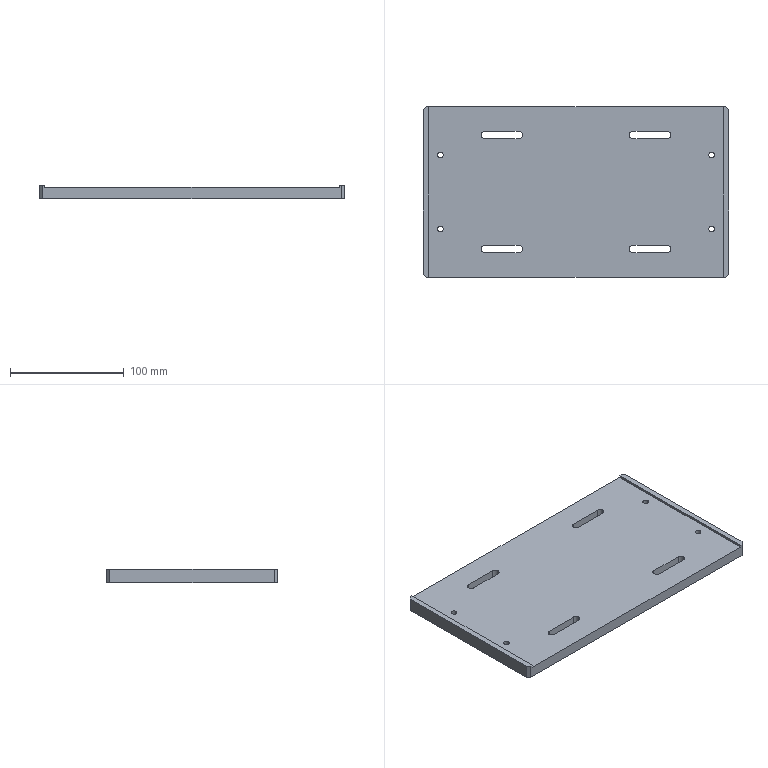Part | SolidWorks | features ICE 2, Chamfer 1, Extrusion 1, HoleWzd 1 | 1 solid | 42 faces | box 268 x 150 x 12 mm | volume 394710 mm3 | plane 22 | cylinder 20 | commonest cylinder face diameters 6.6 x12 5 x8
STEP:
#1=CARTESIAN_POINT('',(-121.5,32.5,0.));
#2=VERTEX_POINT('',#1);
#3=CARTESIAN_POINT('',(-116.5,32.5,0.));
#4=VERTEX_POINT('',#3);
#5=CARTESIAN_POINT('',(-119.,32.5,0.));
#6=DIRECTION('',(0.,0.,1.));
#7=DIRECTION('',(1.,0.,0.));
#8=AXIS2_PLACEMENT_3D('',#5,#6,#7);
#9=CIRCLE('',#8,2.5);
#10=EDGE_CURVE('',#2,#4,#9,.T.);
#11=ORIENTED_EDGE('',*,*,#10,.F.);
#12=CARTESIAN_POINT('',(-121.5,32.5,10.));
#13=VERTEX_POINT('',#12);
#14=CARTESIAN_POINT('',(-121.5,32.5,10.));
#15=DIRECTION('',(0.,0.,1.));
#16=VECTOR('',#15,1000.);
#17=LINE('',#14,#16);
#18=EDGE_CURVE('',#2,#13,#17,.T.);
#19=ORIENTED_EDGE('',*,*,#18,.T.);
#20=CARTESIAN_POINT('',(-116.5,32.5,10.));
#21=VERTEX_POINT('',#20);
#22=CARTESIAN_POINT('',(-119.,32.5,10.));
#23=DIRECTION('',(0.,0.,1.));
#24=DIRECTION('',(1.,0.,0.));
#25=AXIS2_PLACEMENT_3D('',#22,#23,#24);
#26=CIRCLE('',#25,2.5);
#27=EDGE_CURVE('',#13,#21,#26,.T.);
#28=ORIENTED_EDGE('',*,*,#27,.T.);
#29=CARTESIAN_POINT('',(-116.5,32.5,10.));
#30=DIRECTION('',(0.,0.,1.));
#31=VECTOR('',#30,1000.);
#32=LINE('',#29,#31);
#33=EDGE_CURVE('',#4,#21,#32,.T.);
#34=ORIENTED_EDGE('',*,*,#33,.F.);
#35=EDGE_LOOP('',(#11,#19,#28,#34));
#36=FACE_OUTER_BOUND('',#35,.T.);
#37=CARTESIAN_POINT('',(-119.,32.5,10.));
#38=DIRECTION('',(0.,0.,1.));
#39=DIRECTION('',(1.,0.,0.));
#40=AXIS2_PLACEMENT_3D('',#37,#38,#39);
#41=CYLINDRICAL_SURFACE('',#40,2.5);
#42=ADVANCED_FACE('',(#36),#41,.F.);
#43=CARTESIAN_POINT('',(-121.5,-32.5,0.));
#44=VERTEX_POINT('',#43);
#45=CARTESIAN_POINT('',(-116.5,-32.5,0.));
#46=VERTEX_POINT('',#45);
#47=CARTESIAN_POINT('',(-119.,-32.5,0.));
#48=DIRECTION('',(0.,0.,1.));
#49=DIRECTION('',(1.,0.,0.));
#50=AXIS2_PLACEMENT_3D('',#47,#48,#49);
#51=CIRCLE('',#50,2.5);
#52=EDGE_CURVE('',#44,#46,#51,.T.);
#53=ORIENTED_EDGE('',*,*,#52,.F.);
#54=CARTESIAN_POINT('',(-121.5,-32.5,10.));
#55=VERTEX_POINT('',#54);
#56=CARTESIAN_POINT('',(-121.5,-32.5,10.));
#57=DIRECTION('',(0.,0.,1.));
#58=VECTOR('',#57,1000.);
#59=LINE('',#56,#58);
#60=EDGE_CURVE('',#44,#55,#59,.T.);
#61=ORIENTED_EDGE('',*,*,#60,.T.);
#62=CARTESIAN_POINT('',(-116.5,-32.5,10.));
#63=VERTEX_POINT('',#62);
#64=CARTESIAN_POINT('',(-119.,-32.5,10.));
#65=DIRECTION('',(0.,0.,1.));
#66=DIRECTION('',(1.,0.,0.));
#67=AXIS2_PLACEMENT_3D('',#64,#65,#66);
#68=CIRCLE('',#67,2.5);
#69=EDGE_CURVE('',#55,#63,#68,.T.);
#70=ORIENTED_EDGE('',*,*,#69,.T.);
#71=CARTESIAN_POINT('',(-116.5,-32.5,10.));
#72=DIRECTION('',(0.,0.,1.));
#73=VECTOR('',#72,1000.);
#74=LINE('',#71,#73);
#75=EDGE_CURVE('',#46,#63,#74,.T.);
#76=ORIENTED_EDGE('',*,*,#75,.F.);
#77=EDGE_LOOP('',(#53,#61,#70,#76));
#78=FACE_OUTER_BOUND('',#77,.T.);
#79=CARTESIAN_POINT('',(-119.,-32.5,10.));
#80=DIRECTION('',(0.,0.,1.));
#81=DIRECTION('',(1.,0.,0.));
#82=AXIS2_PLACEMENT_3D('',#79,#80,#81);
#83=CYLINDRICAL_SURFACE('',#82,2.5);
#84=ADVANCED_FACE('',(#78),#83,.F.);
#85=CARTESIAN_POINT('',(116.5,32.5,0.));
#86=VERTEX_POINT('',#85);
#87=CARTESIAN_POINT('',(121.5,32.5,0.));
#88=VERTEX_POINT('',#87);
#89=CARTESIAN_POINT('',(119.,32.5,0.));
#90=DIRECTION('',(0.,0.,1.));
#91=DIRECTION('',(1.,0.,0.));
#92=AXIS2_PLACEMENT_3D('',#89,#90,#91);
#93=CIRCLE('',#92,2.5);
#94=EDGE_CURVE('',#86,#88,#93,.T.);
#95=ORIENTED_EDGE('',*,*,#94,.F.);
#96=CARTESIAN_POINT('',(116.5,32.5,10.));
#97=VERTEX_POINT('',#96);
#98=CARTESIAN_POINT('',(116.5,32.5,10.));
#99=DIRECTION('',(0.,0.,1.));
#100=VECTOR('',#99,1000.);
#101=LINE('',#98,#100);
#102=EDGE_CURVE('',#86,#97,#101,.T.);
#103=ORIENTED_EDGE('',*,*,#102,.T.);
#104=CARTESIAN_POINT('',(121.5,32.5,10.));
#105=VERTEX_POINT('',#104);
#106=CARTESIAN_POINT('',(119.,32.5,10.));
#107=DIRECTION('',(0.,0.,1.));
#108=DIRECTION('',(1.,0.,0.));
#109=AXIS2_PLACEMENT_3D('',#106,#107,#108);
#110=CIRCLE('',#109,2.5);
#111=EDGE_CURVE('',#97,#105,#110,.T.);
#112=ORIENTED_EDGE('',*,*,#111,.T.);
#113=CARTESIAN_POINT('',(121.5,32.5,10.));
#114=DIRECTION('',(0.,0.,1.));
#115=VECTOR('',#114,1000.);
#116=LINE('',#113,#115);
#117=EDGE_CURVE('',#88,#105,#116,.T.);
#118=ORIENTED_EDGE('',*,*,#117,.F.);
#119=EDGE_LOOP('',(#95,#103,#112,#118));
#120=FACE_OUTER_BOUND('',#119,.T.);
#121=CARTESIAN_POINT('',(119.,32.5,10.));
#122=DIRECTION('',(0.,0.,1.));
#123=DIRECTION('',(1.,0.,0.));
#124=AXIS2_PLACEMENT_3D('',#121,#122,#123);
#125=CYLINDRICAL_SURFACE('',#124,2.5);
#126=ADVANCED_FACE('',(#120),#125,.F.);
#127=CARTESIAN_POINT('',(116.5,-32.5,0.));
#128=VERTEX_POINT('',#127);
#129=CARTESIAN_POINT('',(121.5,-32.5,0.));
#130=VERTEX_POINT('',#129);
#131=CARTESIAN_POINT('',(119.,-32.5,0.));
#132=DIRECTION('',(0.,0.,1.));
#133=DIRECTION('',(1.,0.,0.));
#134=AXIS2_PLACEMENT_3D('',#131,#132,#133);
#135=CIRCLE('',#134,2.5);
#136=EDGE_CURVE('',#128,#130,#135,.T.);
#137=ORIENTED_EDGE('',*,*,#136,.F.);
#138=CARTESIAN_POINT('',(116.5,-32.5,10.));
#139=VERTEX_POINT('',#138);
#140=CARTESIAN_POINT('',(116.5,-32.5,10.));
#141=DIRECTION('',(0.,0.,1.));
#142=VECTOR('',#141,1000.);
#143=LINE('',#140,#142);
#144=EDGE_CURVE('',#128,#139,#143,.T.);
#145=ORIENTED_EDGE('',*,*,#144,.T.);
#146=CARTESIAN_POINT('',(121.5,-32.5,10.));
#147=VERTEX_POINT('',#146);
#148=CARTESIAN_POINT('',(119.,-32.5,10.));
#149=DIRECTION('',(0.,0.,1.));
#150=DIRECTION('',(1.,0.,0.));
#151=AXIS2_PLACEMENT_3D('',#148,#149,#150);
#152=CIRCLE('',#151,2.5);
#153=EDGE_CURVE('',#139,#147,#152,.T.);
#154=ORIENTED_EDGE('',*,*,#153,.T.);
#155=CARTESIAN_POINT('',(121.5,-32.5,10.));
#156=DIRECTION('',(0.,0.,1.));
#157=VECTOR('',#156,1000.);
#158=LINE('',#155,#157);
#159=EDGE_CURVE('',#130,#147,#158,.T.);
#160=ORIENTED_EDGE('',*,*,#159,.F.);
#161=EDGE_LOOP('',(#137,#145,#154,#160));
#162=FACE_OUTER_BOUND('',#161,.T.);
#163=CARTESIAN_POINT('',(119.,-32.5,10.));
#164=DIRECTION('',(0.,0.,1.));
#165=DIRECTION('',(1.,0.,0.));
#166=AXIS2_PLACEMENT_3D('',#163,#164,#165);
#167=CYLINDRICAL_SURFACE('',#166,2.5);
#168=ADVANCED_FACE('',(#162),#167,.F.);
#169=CARTESIAN_POINT('',(83.3,50.,0.));
#170=VERTEX_POINT('',#169);
#171=CARTESIAN_POINT('',(80.,53.3,0.));
#172=VERTEX_POINT('',#171);
#173=CARTESIAN_POINT('',(80.,50.,0.));
#174=DIRECTION('',(0.,0.,1.));
#175=DIRECTION('',(1.,0.,0.));
#176=AXIS2_PLACEMENT_3D('',#173,#174,#175);
#177=CIRCLE('',#176,3.3);
#178=EDGE_CURVE('',#170,#172,#177,.T.);
#179=ORIENTED_EDGE('',*,*,#178,.F.);
#180=CARTESIAN_POINT('',(83.3,50.,10.));
#181=VERTEX_POINT('',#180);
#182=CARTESIAN_POINT('',(83.3,50.,0.));
#183=DIRECTION('',(0.,0.,1.));
#184=VECTOR('',#183,1000.);
#185=LINE('',#182,#184);
#186=EDGE_CURVE('',#170,#181,#185,.T.);
#187=ORIENTED_EDGE('',*,*,#186,.T.);
#188=CARTESIAN_POINT('',(80.,53.3,10.));
#189=VERTEX_POINT('',#188);
#190=CARTESIAN_POINT('',(80.,50.,10.));
#191=DIRECTION('',(0.,0.,1.));
#192=DIRECTION('',(1.,0.,0.));
#193=AXIS2_PLACEMENT_3D('',#190,#191,#192);
#194=CIRCLE('',#193,3.3);
#195=EDGE_CURVE('',#181,#189,#194,.T.);
#196=ORIENTED_EDGE('',*,*,#195,.T.);
#197=CARTESIAN_POINT('',(80.,53.3,0.));
#198=DIRECTION('',(0.,0.,1.));
#199=VECTOR('',#198,1000.);
#200=LINE('',#197,#199);
#201=EDGE_CURVE('',#172,#189,#200,.T.);
#202=ORIENTED_EDGE('',*,*,#201,.F.);
#203=EDGE_LOOP('',(#179,#187,#196,#202));
#204=FACE_OUTER_BOUND('',#203,.T.);
#205=CARTESIAN_POINT('',(80.,50.,0.));
#206=DIRECTION('',(0.,0.,1.));
#207=DIRECTION('',(1.,0.,0.));
#208=AXIS2_PLACEMENT_3D('',#205,#206,#207);
#209=CYLINDRICAL_SURFACE('',#208,3.3);
#210=ADVANCED_FACE('',(#204),#209,.F.);
#211=CARTESIAN_POINT('',(-46.7,-50.,0.));
#212=VERTEX_POINT('',#211);
#213=CARTESIAN_POINT('',(-50.,-46.7,0.));
#214=VERTEX_POINT('',#213);
#215=CARTESIAN_POINT('',(-50.,-50.,0.));
#216=DIRECTION('',(0.,0.,1.));
#217=DIRECTION('',(1.,0.,0.));
#218=AXIS2_PLACEMENT_3D('',#215,#216,#217);
#219=CIRCLE('',#218,3.3);
#220=EDGE_CURVE('',#212,#214,#219,.T.);
#221=ORIENTED_EDGE('',*,*,#220,.F.);
#222=CARTESIAN_POINT('',(-46.7,-50.,10.));
#223=VERTEX_POINT('',#222);
#224=CARTESIAN_POINT('',(-46.7,-50.,0.));
#225=DIRECTION('',(0.,0.,1.));
#226=VECTOR('',#225,1000.);
#227=LINE('',#224,#226);
#228=EDGE_CURVE('',#212,#223,#227,.T.);
#229=ORIENTED_EDGE('',*,*,#228,.T.);
#230=CARTESIAN_POINT('',(-50.,-46.7,10.));
#231=VERTEX_POINT('',#230);
#232=CARTESIAN_POINT('',(-50.,-50.,10.));
#233=DIRECTION('',(0.,0.,1.));
#234=DIRECTION('',(1.,0.,0.));
#235=AXIS2_PLACEMENT_3D('',#232,#233,#234);
#236=CIRCLE('',#235,3.3);
#237=EDGE_CURVE('',#223,#231,#236,.T.);
#238=ORIENTED_EDGE('',*,*,#237,.T.);
#239=CARTESIAN_POINT('',(-50.,-46.7,0.));
#240=DIRECTION('',(0.,0.,1.));
#241=VECTOR('',#240,1000.);
#242=LINE('',#239,#241);
#243=EDGE_CURVE('',#214,#231,#242,.T.);
#244=ORIENTED_EDGE('',*,*,#243,.F.);
#245=EDGE_LOOP('',(#221,#229,#238,#244));
#246=FACE_OUTER_BOUND('',#245,.T.);
#247=CARTESIAN_POINT('',(-50.,-50.,0.));
#248=DIRECTION('',(0.,0.,1.));
#249=DIRECTION('',(1.,0.,0.));
#250=AXIS2_PLACEMENT_3D('',#247,#248,#249);
#251=CYLINDRICAL_SURFACE('',#250,3.3);
#252=ADVANCED_FACE('',(#246),#251,.F.);
#253=CARTESIAN_POINT('',(83.3,-50.,0.));
#254=VERTEX_POINT('',#253);
#255=CARTESIAN_POINT('',(80.,-46.7,0.));
#256=VERTEX_POINT('',#255);
#257=CARTESIAN_POINT('',(80.,-50.,0.));
#258=DIRECTION('',(0.,0.,1.));
#259=DIRECTION('',(1.,0.,0.));
#260=AXIS2_PLACEMENT_3D('',#257,#258,#259);
#261=CIRCLE('',#260,3.3);
#262=EDGE_CURVE('',#254,#256,#261,.T.);
#263=ORIENTED_EDGE('',*,*,#262,.F.);
#264=CARTESIAN_POINT('',(83.3,-50.,10.));
#265=VERTEX_POINT('',#264);
#266=CARTESIAN_POINT('',(83.3,-50.,0.));
#267=DIRECTION('',(0.,0.,1.));
#268=VECTOR('',#267,1000.);
#269=LINE('',#266,#268);
#270=EDGE_CURVE('',#254,#265,#269,.T.);
#271=ORIENTED_EDGE('',*,*,#270,.T.);
#272=CARTESIAN_POINT('',(80.,-46.7,10.));
#273=VERTEX_POINT('',#272);
#274=CARTESIAN_POINT('',(80.,-50.,10.));
#275=DIRECTION('',(0.,0.,1.));
#276=DIRECTION('',(1.,0.,0.));
#277=AXIS2_PLACEMENT_3D('',#274,#275,#276);
#278=CIRCLE('',#277,3.3);
#279=EDGE_CURVE('',#265,#273,#278,.T.);
#280=ORIENTED_EDGE('',*,*,#279,.T.);
#281=CARTESIAN_POINT('',(80.,-46.7,0.));
#282=DIRECTION('',(0.,0.,1.));
#283=VECTOR('',#282,1000.);
#284=LINE('',#281,#283);
#285=EDGE_CURVE('',#256,#273,#284,.T.);
#286=ORIENTED_EDGE('',*,*,#285,.F.);
#287=EDGE_LOOP('',(#263,#271,#280,#286));
#288=FACE_OUTER_BOUND('',#287,.T.);
#289=CARTESIAN_POINT('',(80.,-50.,0.));
#290=DIRECTION('',(0.,0.,1.));
#291=DIRECTION('',(1.,0.,0.));
#292=AXIS2_PLACEMENT_3D('',#289,#290,#291);
#293=CYLINDRICAL_SURFACE('',#292,3.3);
#294=ADVANCED_FACE('',(#288),#293,.F.);
#295=CARTESIAN_POINT('',(-46.7,50.,0.));
#296=VERTEX_POINT('',#295);
#297=CARTESIAN_POINT('',(-50.,53.3,0.));
#298=VERTEX_POINT('',#297);
#299=CARTESIAN_POINT('',(-50.,50.,0.));
#300=DIRECTION('',(0.,0.,1.));
#301=DIRECTION('',(1.,0.,0.));
#302=AXIS2_PLACEMENT_3D('',#299,#300,#301);
#303=CIRCLE('',#302,3.3);
#304=EDGE_CURVE('',#296,#298,#303,.T.);
#305=ORIENTED_EDGE('',*,*,#304,.F.);
#306=CARTESIAN_POINT('',(-46.7,50.,10.));
#307=VERTEX_POINT('',#306);
#308=CARTESIAN_POINT('',(-46.7,50.,0.));
#309=DIRECTION('',(0.,0.,1.));
#310=VECTOR('',#309,1000.);
#311=LINE('',#308,#310);
#312=EDGE_CURVE('',#296,#307,#311,.T.);
#313=ORIENTED_EDGE('',*,*,#312,.T.);
#314=CARTESIAN_POINT('',(-50.,53.3,10.));
#315=VERTEX_POINT('',#314);
#316=CARTESIAN_POINT('',(-50.,50.,10.));
#317=DIRECTION('',(0.,0.,1.));
#318=DIRECTION('',(1.,0.,0.));
#319=AXIS2_PLACEMENT_3D('',#316,#317,#318);
#320=CIRCLE('',#319,3.3);
#321=EDGE_CURVE('',#307,#315,#320,.T.);
#322=ORIENTED_EDGE('',*,*,#321,.T.);
#323=CARTESIAN_POINT('',(-50.,53.3,0.));
#324=DIRECTION('',(0.,0.,1.));
#325=VECTOR('',#324,1000.);
#326=LINE('',#323,#325);
#327=EDGE_CURVE('',#298,#315,#326,.T.);
#328=ORIENTED_EDGE('',*,*,#327,.F.);
#329=EDGE_LOOP('',(#305,#313,#322,#328));
#330=FACE_OUTER_BOUND('',#329,.T.);
#331=CARTESIAN_POINT('',(-50.,50.,0.));
#332=DIRECTION('',(0.,0.,1.));
#333=DIRECTION('',(1.,0.,0.));
#334=AXIS2_PLACEMENT_3D('',#331,#332,#333);
#335=CYLINDRICAL_SURFACE('',#334,3.3);
#336=ADVANCED_FACE('',(#330),#335,.F.);
#337=CARTESIAN_POINT('',(134.,-72.,12.));
#338=VERTEX_POINT('',#337);
#339=CARTESIAN_POINT('',(134.,72.,12.));
#340=VERTEX_POINT('',#339);
#341=CARTESIAN_POINT('',(134.,-75.,12.));
#342=DIRECTION('',(0.,1.,0.));
#343=VECTOR('',#342,1000.);
#344=LINE('',#341,#343);
#345=EDGE_CURVE('',#338,#340,#344,.T.);
#346=ORIENTED_EDGE('',*,*,#345,.T.);
#347=CARTESIAN_POINT('',(131.,75.,12.));
#348=VERTEX_POINT('',#347);
#349=CARTESIAN_POINT('',(131.,75.,12.));
#350=DIRECTION('',(-0.7071,0.7071,0.));
#351=VECTOR('',#350,1000.);
#352=LINE('',#349,#351);
#353=EDGE_CURVE('',#340,#348,#352,.T.);
#354=ORIENTED_EDGE('',*,*,#353,.T.);
#355=CARTESIAN_POINT('',(129.,75.,12.));
#356=VERTEX_POINT('',#355);
#357=CARTESIAN_POINT('',(-134.,75.,12.));
#358=DIRECTION('',(-1.,0.,0.));
#359=VECTOR('',#358,1000.);
#360=LINE('',#357,#359);
#361=EDGE_CURVE('',#348,#356,#360,.T.);
#362=ORIENTED_EDGE('',*,*,#361,.T.);
#363=CARTESIAN_POINT('',(129.,-75.,12.));
#364=VERTEX_POINT('',#363);
#365=CARTESIAN_POINT('',(129.,-75.,12.));
#366=DIRECTION('',(0.,1.,0.));
#367=VECTOR('',#366,1000.);
#368=LINE('',#365,#367);
#369=EDGE_CURVE('',#364,#356,#368,.T.);
#370=ORIENTED_EDGE('',*,*,#369,.F.);
#371=CARTESIAN_POINT('',(131.,-75.,12.));
#372=VERTEX_POINT('',#371);
#373=CARTESIAN_POINT('',(-134.,-75.,12.));
#374=DIRECTION('',(1.,0.,0.));
#375=VECTOR('',#374,1000.);
#376=LINE('',#373,#375);
#377=EDGE_CURVE('',#364,#372,#376,.T.);
#378=ORIENTED_EDGE('',*,*,#377,.T.);
#379=CARTESIAN_POINT('',(134.,-72.,12.));
#380=DIRECTION('',(0.7071,0.7071,0.));
#381=VECTOR('',#380,1000.);
#382=LINE('',#379,#381);
#383=EDGE_CURVE('',#372,#338,#382,.T.);
#384=ORIENTED_EDGE('',*,*,#383,.T.);
#385=EDGE_LOOP('',(#346,#354,#362,#370,#378,#384));
#386=FACE_OUTER_BOUND('',#385,.T.);
#387=CARTESIAN_POINT('',(0.,0.,12.));
#388=DIRECTION('',(0.,0.,-1.));
#389=DIRECTION('',(-1.,0.,0.));
#390=AXIS2_PLACEMENT_3D('',#387,#388,#389);
#391=PLANE('',#390);
#392=ADVANCED_FACE('',(#386),#391,.F.);
#393=CARTESIAN_POINT('',(134.,-72.,0.));
#394=VERTEX_POINT('',#393);
#395=CARTESIAN_POINT('',(134.,72.,0.));
#396=VERTEX_POINT('',#395);
#397=CARTESIAN_POINT('',(134.,-75.,0.));
#398=DIRECTION('',(0.,1.,0.));
#399=VECTOR('',#398,1000.);
#400=LINE('',#397,#399);
#401=EDGE_CURVE('',#394,#396,#400,.T.);
#402=ORIENTED_EDGE('',*,*,#401,.T.);
#403=CARTESIAN_POINT('',(134.,72.,12.));
#404=DIRECTION('',(0.,0.,1.));
#405=VECTOR('',#404,1000.);
#406=LINE('',#403,#405);
#407=EDGE_CURVE('',#396,#340,#406,.T.);
#408=ORIENTED_EDGE('',*,*,#407,.T.);
#409=ORIENTED_EDGE('',*,*,#345,.F.);
#410=CARTESIAN_POINT('',(134.,-72.,12.));
#411=DIRECTION('',(0.,0.,-1.));
#412=VECTOR('',#411,1000.);
#413=LINE('',#410,#412);
#414=EDGE_CURVE('',#338,#394,#413,.T.);
#415=ORIENTED_EDGE('',*,*,#414,.T.);
#416=EDGE_LOOP('',(#402,#408,#409,#415));
#417=FACE_OUTER_BOUND('',#416,.T.);
#418=CARTESIAN_POINT('',(134.,-75.,12.));
#419=DIRECTION('',(-1.,0.,0.));
#420=DIRECTION('',(0.,0.,1.));
#421=AXIS2_PLACEMENT_3D('',#418,#419,#420);
#422=PLANE('',#421);
#423=ADVANCED_FACE('',(#417),#422,.F.);
#424=CARTESIAN_POINT('',(131.,75.,0.));
#425=VERTEX_POINT('',#424);
#426=CARTESIAN_POINT('',(-131.,75.,0.));
#427=VERTEX_POINT('',#426);
#428=CARTESIAN_POINT('',(-134.,75.,0.));
#429=DIRECTION('',(-1.,0.,0.));
#430=VECTOR('',#429,1000.);
#431=LINE('',#428,#430);
#432=EDGE_CURVE('',#425,#427,#431,.T.);
#433=ORIENTED_EDGE('',*,*,#432,.T.);
#434=CARTESIAN_POINT('',(-131.,75.,12.));
#435=VERTEX_POINT('',#434);
#436=CARTESIAN_POINT('',(-131.,75.,12.));
#437=DIRECTION('',(0.,0.,1.));
#438=VECTOR('',#437,1000.);
#439=LINE('',#436,#438);
#440=EDGE_CURVE('',#427,#435,#439,.T.);
#441=ORIENTED_EDGE('',*,*,#440,.T.);
#442=CARTESIAN_POINT('',(-129.,75.,12.));
#443=VERTEX_POINT('',#442);
#444=CARTESIAN_POINT('',(-134.,75.,12.));
#445=DIRECTION('',(-1.,0.,0.));
#446=VECTOR('',#445,1000.);
#447=LINE('',#444,#446);
#448=EDGE_CURVE('',#443,#435,#447,.T.);
#449=ORIENTED_EDGE('',*,*,#448,.F.);
#450=CARTESIAN_POINT('',(-129.,75.,10.));
#451=VERTEX_POINT('',#450);
#452=CARTESIAN_POINT('',(-129.,75.,10.));
#453=DIRECTION('',(0.,0.,1.));
#454=VECTOR('',#453,1000.);
#455=LINE('',#452,#454);
#456=EDGE_CURVE('',#451,#443,#455,.T.);
#457=ORIENTED_EDGE('',*,*,#456,.F.);
#458=CARTESIAN_POINT('',(129.,75.,10.));
#459=VERTEX_POINT('',#458);
#460=CARTESIAN_POINT('',(-129.,75.,10.));
#461=DIRECTION('',(-1.,0.,0.));
#462=VECTOR('',#461,1000.);
#463=LINE('',#460,#462);
#464=EDGE_CURVE('',#459,#451,#463,.T.);
#465=ORIENTED_EDGE('',*,*,#464,.F.);
#466=CARTESIAN_POINT('',(129.,75.,10.));
#467=DIRECTION('',(0.,0.,1.));
#468=VECTOR('',#467,1000.);
#469=LINE('',#466,#468);
#470=EDGE_CURVE('',#459,#356,#469,.T.);
#471=ORIENTED_EDGE('',*,*,#470,.T.);
#472=ORIENTED_EDGE('',*,*,#361,.F.);
#473=CARTESIAN_POINT('',(131.,75.,12.));
#474=DIRECTION('',(0.,0.,-1.));
#475=VECTOR('',#474,1000.);
#476=LINE('',#473,#475);
#477=EDGE_CURVE('',#348,#425,#476,.T.);
#478=ORIENTED_EDGE('',*,*,#477,.T.);
#479=EDGE_LOOP('',(#433,#441,#449,#457,#465,#471,#472,#478));
#480=FACE_OUTER_BOUND('',#479,.T.);
#481=CARTESIAN_POINT('',(-134.,75.,12.));
#482=DIRECTION('',(0.,-1.,0.));
#483=DIRECTION('',(0.,0.,-1.));
#484=AXIS2_PLACEMENT_3D('',#481,#482,#483);
#485=PLANE('',#484);
#486=ADVANCED_FACE('',(#480),#485,.F.);
#487=CARTESIAN_POINT('',(-134.,72.,12.));
#488=VERTEX_POINT('',#487);
#489=CARTESIAN_POINT('',(-134.,-72.,12.));
#490=VERTEX_POINT('',#489);
#491=CARTESIAN_POINT('',(-134.,-75.,12.));
#492=DIRECTION('',(0.,-1.,0.));
#493=VECTOR('',#492,1000.);
#494=LINE('',#491,#493);
#495=EDGE_CURVE('',#488,#490,#494,.T.);
#496=ORIENTED_EDGE('',*,*,#495,.F.);
#497=CARTESIAN_POINT('',(-134.,72.,0.));
#498=VERTEX_POINT('',#497);
#499=CARTESIAN_POINT('',(-134.,72.,12.));
#500=DIRECTION('',(0.,0.,-1.));
#501=VECTOR('',#500,1000.);
#502=LINE('',#499,#501);
#503=EDGE_CURVE('',#488,#498,#502,.T.);
#504=ORIENTED_EDGE('',*,*,#503,.T.);
#505=CARTESIAN_POINT('',(-134.,-72.,0.));
#506=VERTEX_POINT('',#505);
#507=CARTESIAN_POINT('',(-134.,-75.,0.));
#508=DIRECTION('',(0.,-1.,0.));
#509=VECTOR('',#508,1000.);
#510=LINE('',#507,#509);
#511=EDGE_CURVE('',#498,#506,#510,.T.);
#512=ORIENTED_EDGE('',*,*,#511,.T.);
#513=CARTESIAN_POINT('',(-134.,-72.,12.));
#514=DIRECTION('',(0.,0.,1.));
#515=VECTOR('',#514,1000.);
#516=LINE('',#513,#515);
#517=EDGE_CURVE('',#506,#490,#516,.T.);
#518=ORIENTED_EDGE('',*,*,#517,.T.);
#519=EDGE_LOOP('',(#496,#504,#512,#518));
#520=FACE_OUTER_BOUND('',#519,.T.);
#521=CARTESIAN_POINT('',(-134.,-75.,12.));
#522=DIRECTION('',(1.,0.,0.));
#523=DIRECTION('',(0.,0.,-1.));
#524=AXIS2_PLACEMENT_3D('',#521,#522,#523);
#525=PLANE('',#524);
#526=ADVANCED_FACE('',(#520),#525,.F.);
#527=CARTESIAN_POINT('',(-131.,-75.,0.));
#528=VERTEX_POINT('',#527);
#529=CARTESIAN_POINT('',(131.,-75.,0.));
#530=VERTEX_POINT('',#529);
#531=CARTESIAN_POINT('',(-134.,-75.,0.));
#532=DIRECTION('',(1.,0.,0.));
#533=VECTOR('',#532,1000.);
#534=LINE('',#531,#533);
#535=EDGE_CURVE('',#528,#530,#534,.T.);
#536=ORIENTED_EDGE('',*,*,#535,.T.);
#537=CARTESIAN_POINT('',(131.,-75.,12.));
#538=DIRECTION('',(0.,0.,1.));
#539=VECTOR('',#538,1000.);
#540=LINE('',#537,#539);
#541=EDGE_CURVE('',#530,#372,#540,.T.);
#542=ORIENTED_EDGE('',*,*,#541,.T.);
#543=ORIENTED_EDGE('',*,*,#377,.F.);
#544=CARTESIAN_POINT('',(129.,-75.,10.));
#545=VERTEX_POINT('',#544);
#546=CARTESIAN_POINT('',(129.,-75.,10.));
#547=DIRECTION('',(0.,0.,1.));
#548=VECTOR('',#547,1000.);
#549=LINE('',#546,#548);
#550=EDGE_CURVE('',#545,#364,#549,.T.);
#551=ORIENTED_EDGE('',*,*,#550,.F.);
#552=CARTESIAN_POINT('',(-129.,-75.,10.));
#553=VERTEX_POINT('',#552);
#554=CARTESIAN_POINT('',(-129.,-75.,10.));
#555=DIRECTION('',(1.,0.,0.));
#556=VECTOR('',#555,1000.);
#557=LINE('',#554,#556);
#558=EDGE_CURVE('',#553,#545,#557,.T.);
#559=ORIENTED_EDGE('',*,*,#558,.F.);
#560=CARTESIAN_POINT('',(-129.,-75.,12.));
#561=VERTEX_POINT('',#560);
#562=CARTESIAN_POINT('',(-129.,-75.,10.));
#563=DIRECTION('',(0.,0.,1.));
#564=VECTOR('',#563,1000.);
#565=LINE('',#562,#564);
#566=EDGE_CURVE('',#553,#561,#565,.T.);
#567=ORIENTED_EDGE('',*,*,#566,.T.);
#568=CARTESIAN_POINT('',(-131.,-75.,12.));
#569=VERTEX_POINT('',#568);
#570=CARTESIAN_POINT('',(-134.,-75.,12.));
#571=DIRECTION('',(1.,0.,0.));
#572=VECTOR('',#571,1000.);
#573=LINE('',#570,#572);
#574=EDGE_CURVE('',#569,#561,#573,.T.);
#575=ORIENTED_EDGE('',*,*,#574,.F.);
#576=CARTESIAN_POINT('',(-131.,-75.,12.));
#577=DIRECTION('',(0.,0.,-1.));
#578=VECTOR('',#577,1000.);
#579=LINE('',#576,#578);
#580=EDGE_CURVE('',#569,#528,#579,.T.);
#581=ORIENTED_EDGE('',*,*,#580,.T.);
#582=EDGE_LOOP('',(#536,#542,#543,#551,#559,#567,#575,#581));
#583=FACE_OUTER_BOUND('',#582,.T.);
#584=CARTESIAN_POINT('',(-134.,-75.,12.));
#585=DIRECTION('',(0.,1.,0.));
#586=DIRECTION('',(0.,0.,1.));
#587=AXIS2_PLACEMENT_3D('',#584,#585,#586);
#588=PLANE('',#587);
#589=ADVANCED_FACE('',(#583),#588,.F.);
#590=ORIENTED_EDGE('',*,*,#448,.T.);
#591=CARTESIAN_POINT('',(-134.,72.,12.));
#592=DIRECTION('',(-0.7071,-0.7071,0.));
#593=VECTOR('',#592,1000.);
#594=LINE('',#591,#593);
#595=EDGE_CURVE('',#435,#488,#594,.T.);
#596=ORIENTED_EDGE('',*,*,#595,.T.);
#597=ORIENTED_EDGE('',*,*,#495,.T.);
#598=CARTESIAN_POINT('',(-131.,-75.,12.));
#599=DIRECTION('',(0.7071,-0.7071,0.));
#600=VECTOR('',#599,1000.);
#601=LINE('',#598,#600);
#602=EDGE_CURVE('',#490,#569,#601,.T.);
#603=ORIENTED_EDGE('',*,*,#602,.T.);
#604=ORIENTED_EDGE('',*,*,#574,.T.);
#605=CARTESIAN_POINT('',(-129.,-75.,12.));
#606=DIRECTION('',(0.,-1.,0.));
#607=VECTOR('',#606,1000.);
#608=LINE('',#605,#607);
#609=EDGE_CURVE('',#443,#561,#608,.T.);
#610=ORIENTED_EDGE('',*,*,#609,.F.);
#611=EDGE_LOOP('',(#590,#596,#597,#603,#604,#610));
#612=FACE_OUTER_BOUND('',#611,.T.);
#613=CARTESIAN_POINT('',(0.,0.,12.));
#614=DIRECTION('',(0.,0.,-1.));
#615=DIRECTION('',(-1.,0.,0.));
#616=AXIS2_PLACEMENT_3D('',#613,#614,#615);
#617=PLANE('',#616);
#618=ADVANCED_FACE('',(#612),#617,.F.);
#619=CARTESIAN_POINT('',(-119.,32.5,0.));
#620=DIRECTION('',(0.,0.,1.));
#621=DIRECTION('',(1.,0.,0.));
#622=AXIS2_PLACEMENT_3D('',#619,#620,#621);
#623=CIRCLE('',#622,2.5);
#624=EDGE_CURVE('',#4,#2,#623,.T.);
#625=ORIENTED_EDGE('',*,*,#624,.T.);
#626=ORIENTED_EDGE('',*,*,#10,.T.);
#627=EDGE_LOOP('',(#625,#626));
#628=FACE_BOUND('',#627,.T.);
#629=CARTESIAN_POINT('',(-119.,-32.5,0.));
#630=DIRECTION('',(0.,0.,1.));
#631=DIRECTION('',(1.,0.,0.));
#632=AXIS2_PLACEMENT_3D('',#629,#630,#631);
#633=CIRCLE('',#632,2.5);
#634=EDGE_CURVE('',#46,#44,#633,.T.);
#635=ORIENTED_EDGE('',*,*,#634,.T.);
#636=ORIENTED_EDGE('',*,*,#52,.T.);
#637=EDGE_LOOP('',(#635,#636));
#638=FACE_BOUND('',#637,.T.);
#639=CARTESIAN_POINT('',(119.,32.5,0.));
#640=DIRECTION('',(0.,0.,1.));
#641=DIRECTION('',(1.,0.,0.));
#642=AXIS2_PLACEMENT_3D('',#639,#640,#641);
#643=CIRCLE('',#642,2.5);
#644=EDGE_CURVE('',#88,#86,#643,.T.);
#645=ORIENTED_EDGE('',*,*,#644,.T.);
#646=ORIENTED_EDGE('',*,*,#94,.T.);
#647=EDGE_LOOP('',(#645,#646));
#648=FACE_BOUND('',#647,.T.);
#649=CARTESIAN_POINT('',(119.,-32.5,0.));
#650=DIRECTION('',(0.,0.,1.));
#651=DIRECTION('',(1.,0.,0.));
#652=AXIS2_PLACEMENT_3D('',#649,#650,#651);
#653=CIRCLE('',#652,2.5);
#654=EDGE_CURVE('',#130,#128,#653,.T.);
#655=ORIENTED_EDGE('',*,*,#654,.T.);
#656=ORIENTED_EDGE('',*,*,#136,.T.);
#657=EDGE_LOOP('',(#655,#656));
#658=FACE_BOUND('',#657,.T.);
#659=CARTESIAN_POINT('',(50.,53.3,0.));
#660=VERTEX_POINT('',#659);
#661=CARTESIAN_POINT('',(50.,46.7,0.));
#662=VERTEX_POINT('',#661);
#663=CARTESIAN_POINT('',(50.,50.,0.));
#664=DIRECTION('',(0.,0.,1.));
#665=DIRECTION('',(1.,0.,0.));
#666=AXIS2_PLACEMENT_3D('',#663,#664,#665);
#667=CIRCLE('',#666,3.3);
#668=EDGE_CURVE('',#660,#662,#667,.T.);
#669=ORIENTED_EDGE('',*,*,#668,.T.);
#670=CARTESIAN_POINT('',(80.,46.7,0.));
#671=VERTEX_POINT('',#670);
#672=CARTESIAN_POINT('',(50.,46.7,0.));
#673=DIRECTION('',(1.,0.,0.));
#674=VECTOR('',#673,1000.);
#675=LINE('',#672,#674);
#676=EDGE_CURVE('',#662,#671,#675,.T.);
#677=ORIENTED_EDGE('',*,*,#676,.T.);
#678=CARTESIAN_POINT('',(80.,50.,0.));
#679=DIRECTION('',(0.,0.,1.));
#680=DIRECTION('',(1.,0.,0.));
#681=AXIS2_PLACEMENT_3D('',#678,#679,#680);
#682=CIRCLE('',#681,3.3);
#683=EDGE_CURVE('',#671,#170,#682,.T.);
#684=ORIENTED_EDGE('',*,*,#683,.T.);
#685=ORIENTED_EDGE('',*,*,#178,.T.);
#686=CARTESIAN_POINT('',(50.,53.3,0.));
#687=DIRECTION('',(-1.,0.,0.));
#688=VECTOR('',#687,1000.);
#689=LINE('',#686,#688);
#690=EDGE_CURVE('',#172,#660,#689,.T.);
#691=ORIENTED_EDGE('',*,*,#690,.T.);
#692=EDGE_LOOP('',(#669,#677,#684,#685,#691));
#693=FACE_BOUND('',#692,.T.);
#694=CARTESIAN_POINT('',(-80.,-46.7,0.));
#695=VERTEX_POINT('',#694);
#696=CARTESIAN_POINT('',(-80.,-53.3,0.));
#697=VERTEX_POINT('',#696);
#698=CARTESIAN_POINT('',(-80.,-50.,0.));
#699=DIRECTION('',(0.,0.,1.));
#700=DIRECTION('',(1.,0.,0.));
#701=AXIS2_PLACEMENT_3D('',#698,#699,#700);
#702=CIRCLE('',#701,3.3);
#703=EDGE_CURVE('',#695,#697,#702,.T.);
#704=ORIENTED_EDGE('',*,*,#703,.T.);
#705=CARTESIAN_POINT('',(-50.,-53.3,0.));
#706=VERTEX_POINT('',#705);
#707=CARTESIAN_POINT('',(-80.,-53.3,0.));
#708=DIRECTION('',(1.,0.,0.));
#709=VECTOR('',#708,1000.);
#710=LINE('',#707,#709);
#711=EDGE_CURVE('',#697,#706,#710,.T.);
#712=ORIENTED_EDGE('',*,*,#711,.T.);
#713=CARTESIAN_POINT('',(-50.,-50.,0.));
#714=DIRECTION('',(0.,0.,1.));
#715=DIRECTION('',(1.,0.,0.));
#716=AXIS2_PLACEMENT_3D('',#713,#714,#715);
#717=CIRCLE('',#716,3.3);
#718=EDGE_CURVE('',#706,#212,#717,.T.);
#719=ORIENTED_EDGE('',*,*,#718,.T.);
#720=ORIENTED_EDGE('',*,*,#220,.T.);
#721=CARTESIAN_POINT('',(-80.,-46.7,0.));
#722=DIRECTION('',(-1.,0.,0.));
#723=VECTOR('',#722,1000.);
#724=LINE('',#721,#723);
#725=EDGE_CURVE('',#214,#695,#724,.T.);
#726=ORIENTED_EDGE('',*,*,#725,.T.);
#727=EDGE_LOOP('',(#704,#712,#719,#720,#726));
#728=FACE_BOUND('',#727,.T.);
#729=CARTESIAN_POINT('',(50.,-46.7,0.));
#730=VERTEX_POINT('',#729);
#731=CARTESIAN_POINT('',(50.,-53.3,0.));
#732=VERTEX_POINT('',#731);
#733=CARTESIAN_POINT('',(50.,-50.,0.));
#734=DIRECTION('',(0.,0.,1.));
#735=DIRECTION('',(1.,0.,0.));
#736=AXIS2_PLACEMENT_3D('',#733,#734,#735);
#737=CIRCLE('',#736,3.3);
#738=EDGE_CURVE('',#730,#732,#737,.T.);
#739=ORIENTED_EDGE('',*,*,#738,.T.);
#740=CARTESIAN_POINT('',(80.,-53.3,0.));
#741=VERTEX_POINT('',#740);
#742=CARTESIAN_POINT('',(50.,-53.3,0.));
#743=DIRECTION('',(1.,0.,0.));
#744=VECTOR('',#743,1000.);
#745=LINE('',#742,#744);
#746=EDGE_CURVE('',#732,#741,#745,.T.);
#747=ORIENTED_EDGE('',*,*,#746,.T.);
#748=CARTESIAN_POINT('',(80.,-50.,0.));
#749=DIRECTION('',(0.,0.,1.));
#750=DIRECTION('',(1.,0.,0.));
#751=AXIS2_PLACEMENT_3D('',#748,#749,#750);
#752=CIRCLE('',#751,3.3);
#753=EDGE_CURVE('',#741,#254,#752,.T.);
#754=ORIENTED_EDGE('',*,*,#753,.T.);
#755=ORIENTED_EDGE('',*,*,#262,.T.);
#756=CARTESIAN_POINT('',(50.,-46.7,0.));
#757=DIRECTION('',(-1.,0.,0.));
#758=VECTOR('',#757,1000.);
#759=LINE('',#756,#758);
#760=EDGE_CURVE('',#256,#730,#759,.T.);
#761=ORIENTED_EDGE('',*,*,#760,.T.);
#762=EDGE_LOOP('',(#739,#747,#754,#755,#761));
#763=FACE_BOUND('',#762,.T.);
#764=CARTESIAN_POINT('',(-80.,53.3,0.));
#765=VERTEX_POINT('',#764);
#766=CARTESIAN_POINT('',(-80.,46.7,0.));
#767=VERTEX_POINT('',#766);
#768=CARTESIAN_POINT('',(-80.,50.,0.));
#769=DIRECTION('',(0.,0.,1.));
#770=DIRECTION('',(1.,0.,0.));
#771=AXIS2_PLACEMENT_3D('',#768,#769,#770);
#772=CIRCLE('',#771,3.3);
#773=EDGE_CURVE('',#765,#767,#772,.T.);
#774=ORIENTED_EDGE('',*,*,#773,.T.);
#775=CARTESIAN_POINT('',(-50.,46.7,0.));
#776=VERTEX_POINT('',#775);
#777=CARTESIAN_POINT('',(-80.,46.7,0.));
#778=DIRECTION('',(1.,0.,0.));
#779=VECTOR('',#778,1000.);
#780=LINE('',#777,#779);
#781=EDGE_CURVE('',#767,#776,#780,.T.);
#782=ORIENTED_EDGE('',*,*,#781,.T.);
#783=CARTESIAN_POINT('',(-50.,50.,0.));
#784=DIRECTION('',(0.,0.,1.));
#785=DIRECTION('',(1.,0.,0.));
#786=AXIS2_PLACEMENT_3D('',#783,#784,#785);
#787=CIRCLE('',#786,3.3);
#788=EDGE_CURVE('',#776,#296,#787,.T.);
#789=ORIENTED_EDGE('',*,*,#788,.T.);
#790=ORIENTED_EDGE('',*,*,#304,.T.);
#791=CARTESIAN_POINT('',(-80.,53.3,0.));
#792=DIRECTION('',(-1.,0.,0.));
#793=VECTOR('',#792,1000.);
#794=LINE('',#791,#793);
#795=EDGE_CURVE('',#298,#765,#794,.T.);
#796=ORIENTED_EDGE('',*,*,#795,.T.);
#797=EDGE_LOOP('',(#774,#782,#789,#790,#796));
#798=FACE_BOUND('',#797,.T.);
#799=ORIENTED_EDGE('',*,*,#511,.F.);
#800=CARTESIAN_POINT('',(-103.,103.,0.));
#801=DIRECTION('',(0.7071,0.7071,0.));
#802=VECTOR('',#801,1000.);
#803=LINE('',#800,#802);
#804=EDGE_CURVE('',#498,#427,#803,.T.);
#805=ORIENTED_EDGE('',*,*,#804,.T.);
#806=ORIENTED_EDGE('',*,*,#432,.F.);
#807=CARTESIAN_POINT('',(103.,103.,0.));
#808=DIRECTION('',(0.7071,-0.7071,0.));
#809=VECTOR('',#808,1000.);
#810=LINE('',#807,#809);
#811=EDGE_CURVE('',#425,#396,#810,.T.);
#812=ORIENTED_EDGE('',*,*,#811,.T.);
#813=ORIENTED_EDGE('',*,*,#401,.F.);
#814=CARTESIAN_POINT('',(103.,-103.,0.));
#815=DIRECTION('',(-0.7071,-0.7071,0.));
#816=VECTOR('',#815,1000.);
#817=LINE('',#814,#816);
#818=EDGE_CURVE('',#394,#530,#817,.T.);
#819=ORIENTED_EDGE('',*,*,#818,.T.);
#820=ORIENTED_EDGE('',*,*,#535,.F.);
#821=CARTESIAN_POINT('',(-103.,-103.,0.));
#822=DIRECTION('',(-0.7071,0.7071,0.));
#823=VECTOR('',#822,1000.);
#824=LINE('',#821,#823);
#825=EDGE_CURVE('',#528,#506,#824,.T.);
#826=ORIENTED_EDGE('',*,*,#825,.T.);
#827=EDGE_LOOP('',(#799,#805,#806,#812,#813,#819,#820,#826));
#828=FACE_OUTER_BOUND('',#827,.T.);
#829=CARTESIAN_POINT('',(0.,0.,0.));
#830=DIRECTION('',(0.,0.,-1.));
#831=DIRECTION('',(-1.,0.,0.));
#832=AXIS2_PLACEMENT_3D('',#829,#830,#831);
#833=PLANE('',#832);
#834=ADVANCED_FACE('',(#628,#638,#648,#658,#693,#728,#763,#798,#828),#833,.T.);
#835=ORIENTED_EDGE('',*,*,#369,.T.);
#836=ORIENTED_EDGE('',*,*,#470,.F.);
#837=CARTESIAN_POINT('',(129.,-75.,10.));
#838=DIRECTION('',(0.,1.,0.));
#839=VECTOR('',#838,1000.);
#840=LINE('',#837,#839);
#841=EDGE_CURVE('',#545,#459,#840,.T.);
#842=ORIENTED_EDGE('',*,*,#841,.F.);
#843=ORIENTED_EDGE('',*,*,#550,.T.);
#844=EDGE_LOOP('',(#835,#836,#842,#843));
#845=FACE_OUTER_BOUND('',#844,.T.);
#846=CARTESIAN_POINT('',(129.,-75.,10.));
#847=DIRECTION('',(1.,0.,0.));
#848=DIRECTION('',(0.,0.,-1.));
#849=AXIS2_PLACEMENT_3D('',#846,#847,#848);
#850=PLANE('',#849);
#851=ADVANCED_FACE('',(#845),#850,.F.);
#852=ORIENTED_EDGE('',*,*,#609,.T.);
#853=ORIENTED_EDGE('',*,*,#566,.F.);
#854=CARTESIAN_POINT('',(-129.,-75.,10.));
#855=DIRECTION('',(0.,-1.,0.));
#856=VECTOR('',#855,1000.);
#857=LINE('',#854,#856);
#858=EDGE_CURVE('',#451,#553,#857,.T.);
#859=ORIENTED_EDGE('',*,*,#858,.F.);
#860=ORIENTED_EDGE('',*,*,#456,.T.);
#861=EDGE_LOOP('',(#852,#853,#859,#860));
#862=FACE_OUTER_BOUND('',#861,.T.);
#863=CARTESIAN_POINT('',(-129.,-75.,10.));
#864=DIRECTION('',(-1.,0.,0.));
#865=DIRECTION('',(0.,0.,1.));
#866=AXIS2_PLACEMENT_3D('',#863,#864,#865);
#867=PLANE('',#866);
#868=ADVANCED_FACE('',(#862),#867,.F.);
#869=CARTESIAN_POINT('',(-119.,32.5,10.));
#870=DIRECTION('',(0.,0.,1.));
#871=DIRECTION('',(1.,0.,0.));
#872=AXIS2_PLACEMENT_3D('',#869,#870,#871);
#873=CIRCLE('',#872,2.5);
#874=EDGE_CURVE('',#21,#13,#873,.T.);
#875=ORIENTED_EDGE('',*,*,#874,.F.);
#876=ORIENTED_EDGE('',*,*,#27,.F.);
#877=EDGE_LOOP('',(#875,#876));
#878=FACE_BOUND('',#877,.T.);
#879=CARTESIAN_POINT('',(-119.,-32.5,10.));
#880=DIRECTION('',(0.,0.,1.));
#881=DIRECTION('',(1.,0.,0.));
#882=AXIS2_PLACEMENT_3D('',#879,#880,#881);
#883=CIRCLE('',#882,2.5);
#884=EDGE_CURVE('',#63,#55,#883,.T.);
#885=ORIENTED_EDGE('',*,*,#884,.F.);
#886=ORIENTED_EDGE('',*,*,#69,.F.);
#887=EDGE_LOOP('',(#885,#886));
#888=FACE_BOUND('',#887,.T.);
#889=CARTESIAN_POINT('',(119.,32.5,10.));
#890=DIRECTION('',(0.,0.,1.));
#891=DIRECTION('',(1.,0.,0.));
#892=AXIS2_PLACEMENT_3D('',#889,#890,#891);
#893=CIRCLE('',#892,2.5);
#894=EDGE_CURVE('',#105,#97,#893,.T.);
#895=ORIENTED_EDGE('',*,*,#894,.F.);
#896=ORIENTED_EDGE('',*,*,#111,.F.);
#897=EDGE_LOOP('',(#895,#896));
#898=FACE_BOUND('',#897,.T.);
#899=CARTESIAN_POINT('',(119.,-32.5,10.));
#900=DIRECTION('',(0.,0.,1.));
#901=DIRECTION('',(1.,0.,0.));
#902=AXIS2_PLACEMENT_3D('',#899,#900,#901);
#903=CIRCLE('',#902,2.5);
#904=EDGE_CURVE('',#147,#139,#903,.T.);
#905=ORIENTED_EDGE('',*,*,#904,.F.);
#906=ORIENTED_EDGE('',*,*,#153,.F.);
#907=EDGE_LOOP('',(#905,#906));
#908=FACE_BOUND('',#907,.T.);
#909=CARTESIAN_POINT('',(50.,46.7,10.));
#910=VERTEX_POINT('',#909);
#911=CARTESIAN_POINT('',(80.,46.7,10.));
#912=VERTEX_POINT('',#911);
#913=CARTESIAN_POINT('',(50.,46.7,10.));
#914=DIRECTION('',(1.,0.,0.));
#915=VECTOR('',#914,1000.);
#916=LINE('',#913,#915);
#917=EDGE_CURVE('',#910,#912,#916,.T.);
#918=ORIENTED_EDGE('',*,*,#917,.F.);
#919=CARTESIAN_POINT('',(50.,53.3,10.));
#920=VERTEX_POINT('',#919);
#921=CARTESIAN_POINT('',(50.,50.,10.));
#922=DIRECTION('',(0.,0.,1.));
#923=DIRECTION('',(1.,0.,0.));
#924=AXIS2_PLACEMENT_3D('',#921,#922,#923);
#925=CIRCLE('',#924,3.3);
#926=EDGE_CURVE('',#920,#910,#925,.T.);
#927=ORIENTED_EDGE('',*,*,#926,.F.);
#928=CARTESIAN_POINT('',(50.,53.3,10.));
#929=DIRECTION('',(-1.,0.,0.));
#930=VECTOR('',#929,1000.);
#931=LINE('',#928,#930);
#932=EDGE_CURVE('',#189,#920,#931,.T.);
#933=ORIENTED_EDGE('',*,*,#932,.F.);
#934=ORIENTED_EDGE('',*,*,#195,.F.);
#935=CARTESIAN_POINT('',(80.,50.,10.));
#936=DIRECTION('',(0.,0.,1.));
#937=DIRECTION('',(1.,0.,0.));
#938=AXIS2_PLACEMENT_3D('',#935,#936,#937);
#939=CIRCLE('',#938,3.3);
#940=EDGE_CURVE('',#912,#181,#939,.T.);
#941=ORIENTED_EDGE('',*,*,#940,.F.);
#942=EDGE_LOOP('',(#918,#927,#933,#934,#941));
#943=FACE_BOUND('',#942,.T.);
#944=CARTESIAN_POINT('',(-80.,-53.3,10.));
#945=VERTEX_POINT('',#944);
#946=CARTESIAN_POINT('',(-50.,-53.3,10.));
#947=VERTEX_POINT('',#946);
#948=CARTESIAN_POINT('',(-80.,-53.3,10.));
#949=DIRECTION('',(1.,0.,0.));
#950=VECTOR('',#949,1000.);
#951=LINE('',#948,#950);
#952=EDGE_CURVE('',#945,#947,#951,.T.);
#953=ORIENTED_EDGE('',*,*,#952,.F.);
#954=CARTESIAN_POINT('',(-80.,-46.7,10.));
#955=VERTEX_POINT('',#954);
#956=CARTESIAN_POINT('',(-80.,-50.,10.));
#957=DIRECTION('',(0.,0.,1.));
#958=DIRECTION('',(1.,0.,0.));
#959=AXIS2_PLACEMENT_3D('',#956,#957,#958);
#960=CIRCLE('',#959,3.3);
#961=EDGE_CURVE('',#955,#945,#960,.T.);
#962=ORIENTED_EDGE('',*,*,#961,.F.);
#963=CARTESIAN_POINT('',(-80.,-46.7,10.));
#964=DIRECTION('',(-1.,0.,0.));
#965=VECTOR('',#964,1000.);
#966=LINE('',#963,#965);
#967=EDGE_CURVE('',#231,#955,#966,.T.);
#968=ORIENTED_EDGE('',*,*,#967,.F.);
#969=ORIENTED_EDGE('',*,*,#237,.F.);
#970=CARTESIAN_POINT('',(-50.,-50.,10.));
#971=DIRECTION('',(0.,0.,1.));
#972=DIRECTION('',(1.,0.,0.));
#973=AXIS2_PLACEMENT_3D('',#970,#971,#972);
#974=CIRCLE('',#973,3.3);
#975=EDGE_CURVE('',#947,#223,#974,.T.);
#976=ORIENTED_EDGE('',*,*,#975,.F.);
#977=EDGE_LOOP('',(#953,#962,#968,#969,#976));
#978=FACE_BOUND('',#977,.T.);
#979=CARTESIAN_POINT('',(50.,-53.3,10.));
#980=VERTEX_POINT('',#979);
#981=CARTESIAN_POINT('',(80.,-53.3,10.));
#982=VERTEX_POINT('',#981);
#983=CARTESIAN_POINT('',(50.,-53.3,10.));
#984=DIRECTION('',(1.,0.,0.));
#985=VECTOR('',#984,1000.);
#986=LINE('',#983,#985);
#987=EDGE_CURVE('',#980,#982,#986,.T.);
#988=ORIENTED_EDGE('',*,*,#987,.F.);
#989=CARTESIAN_POINT('',(50.,-46.7,10.));
#990=VERTEX_POINT('',#989);
#991=CARTESIAN_POINT('',(50.,-50.,10.));
#992=DIRECTION('',(0.,0.,1.));
#993=DIRECTION('',(1.,0.,0.));
#994=AXIS2_PLACEMENT_3D('',#991,#992,#993);
#995=CIRCLE('',#994,3.3);
#996=EDGE_CURVE('',#990,#980,#995,.T.);
#997=ORIENTED_EDGE('',*,*,#996,.F.);
#998=CARTESIAN_POINT('',(50.,-46.7,10.));
#999=DIRECTION('',(-1.,0.,0.));
#1000=VECTOR('',#999,1000.);
#1001=LINE('',#998,#1000);
#1002=EDGE_CURVE('',#273,#990,#1001,.T.);
#1003=ORIENTED_EDGE('',*,*,#1002,.F.);
#1004=ORIENTED_EDGE('',*,*,#279,.F.);
#1005=CARTESIAN_POINT('',(80.,-50.,10.));
#1006=DIRECTION('',(0.,0.,1.));
#1007=DIRECTION('',(1.,0.,0.));
#1008=AXIS2_PLACEMENT_3D('',#1005,#1006,#1007);
#1009=CIRCLE('',#1008,3.3);
#1010=EDGE_CURVE('',#982,#265,#1009,.T.);
#1011=ORIENTED_EDGE('',*,*,#1010,.F.);
#1012=EDGE_LOOP('',(#988,#997,#1003,#1004,#1011));
#1013=FACE_BOUND('',#1012,.T.);
#1014=CARTESIAN_POINT('',(-80.,46.7,10.));
#1015=VERTEX_POINT('',#1014);
#1016=CARTESIAN_POINT('',(-50.,46.7,10.));
#1017=VERTEX_POINT('',#1016);
#1018=CARTESIAN_POINT('',(-80.,46.7,10.));
#1019=DIRECTION('',(1.,0.,0.));
#1020=VECTOR('',#1019,1000.);
#1021=LINE('',#1018,#1020);
#1022=EDGE_CURVE('',#1015,#1017,#1021,.T.);
#1023=ORIENTED_EDGE('',*,*,#1022,.F.);
#1024=CARTESIAN_POINT('',(-80.,53.3,10.));
#1025=VERTEX_POINT('',#1024);
#1026=CARTESIAN_POINT('',(-80.,50.,10.));
#1027=DIRECTION('',(0.,0.,1.));
#1028=DIRECTION('',(1.,0.,0.));
#1029=AXIS2_PLACEMENT_3D('',#1026,#1027,#1028);
#1030=CIRCLE('',#1029,3.3);
#1031=EDGE_CURVE('',#1025,#1015,#1030,.T.);
#1032=ORIENTED_EDGE('',*,*,#1031,.F.);
#1033=CARTESIAN_POINT('',(-80.,53.3,10.));
#1034=DIRECTION('',(-1.,0.,0.));
#1035=VECTOR('',#1034,1000.);
#1036=LINE('',#1033,#1035);
#1037=EDGE_CURVE('',#315,#1025,#1036,.T.);
#1038=ORIENTED_EDGE('',*,*,#1037,.F.);
#1039=ORIENTED_EDGE('',*,*,#321,.F.);
#1040=CARTESIAN_POINT('',(-50.,50.,10.));
#1041=DIRECTION('',(0.,0.,1.));
#1042=DIRECTION('',(1.,0.,0.));
#1043=AXIS2_PLACEMENT_3D('',#1040,#1041,#1042);
#1044=CIRCLE('',#1043,3.3);
#1045=EDGE_CURVE('',#1017,#307,#1044,.T.);
#1046=ORIENTED_EDGE('',*,*,#1045,.F.);
#1047=EDGE_LOOP('',(#1023,#1032,#1038,#1039,#1046));
#1048=FACE_BOUND('',#1047,.T.);
#1049=ORIENTED_EDGE('',*,*,#841,.T.);
#1050=ORIENTED_EDGE('',*,*,#464,.T.);
#1051=ORIENTED_EDGE('',*,*,#858,.T.);
#1052=ORIENTED_EDGE('',*,*,#558,.T.);
#1053=EDGE_LOOP('',(#1049,#1050,#1051,#1052));
#1054=FACE_OUTER_BOUND('',#1053,.T.);
#1055=CARTESIAN_POINT('',(0.,0.,10.));
#1056=DIRECTION('',(0.,0.,-1.));
#1057=DIRECTION('',(-1.,0.,0.));
#1058=AXIS2_PLACEMENT_3D('',#1055,#1056,#1057);
#1059=PLANE('',#1058);
#1060=ADVANCED_FACE('',(#878,#888,#898,#908,#943,#978,#1013,#1048,#1054),#1059,.F.);
#1061=ORIENTED_EDGE('',*,*,#1031,.T.);
#1062=CARTESIAN_POINT('',(-80.,46.7,0.));
#1063=DIRECTION('',(0.,0.,1.));
#1064=VECTOR('',#1063,1000.);
#1065=LINE('',#1062,#1064);
#1066=EDGE_CURVE('',#767,#1015,#1065,.T.);
#1067=ORIENTED_EDGE('',*,*,#1066,.F.);
#1068=ORIENTED_EDGE('',*,*,#773,.F.);
#1069=CARTESIAN_POINT('',(-80.,53.3,0.));
#1070=DIRECTION('',(0.,0.,1.));
#1071=VECTOR('',#1070,1000.);
#1072=LINE('',#1069,#1071);
#1073=EDGE_CURVE('',#765,#1025,#1072,.T.);
#1074=ORIENTED_EDGE('',*,*,#1073,.T.);
#1075=EDGE_LOOP('',(#1061,#1067,#1068,#1074));
#1076=FACE_OUTER_BOUND('',#1075,.T.);
#1077=CARTESIAN_POINT('',(-80.,50.,0.));
#1078=DIRECTION('',(0.,0.,1.));
#1079=DIRECTION('',(1.,0.,0.));
#1080=AXIS2_PLACEMENT_3D('',#1077,#1078,#1079);
#1081=CYLINDRICAL_SURFACE('',#1080,3.3);
#1082=ADVANCED_FACE('',(#1076),#1081,.F.);
#1083=ORIENTED_EDGE('',*,*,#1037,.T.);
#1084=ORIENTED_EDGE('',*,*,#1073,.F.);
#1085=ORIENTED_EDGE('',*,*,#795,.F.);
#1086=ORIENTED_EDGE('',*,*,#327,.T.);
#1087=EDGE_LOOP('',(#1083,#1084,#1085,#1086));
#1088=FACE_OUTER_BOUND('',#1087,.T.);
#1089=CARTESIAN_POINT('',(-80.,53.3,0.));
#1090=DIRECTION('',(0.,1.,0.));
#1091=DIRECTION('',(0.,0.,1.));
#1092=AXIS2_PLACEMENT_3D('',#1089,#1090,#1091);
#1093=PLANE('',#1092);
#1094=ADVANCED_FACE('',(#1088),#1093,.F.);
#1095=ORIENTED_EDGE('',*,*,#312,.F.);
#1096=ORIENTED_EDGE('',*,*,#788,.F.);
#1097=CARTESIAN_POINT('',(-50.,46.7,0.));
#1098=DIRECTION('',(0.,0.,1.));
#1099=VECTOR('',#1098,1000.);
#1100=LINE('',#1097,#1099);
#1101=EDGE_CURVE('',#776,#1017,#1100,.T.);
#1102=ORIENTED_EDGE('',*,*,#1101,.T.);
#1103=ORIENTED_EDGE('',*,*,#1045,.T.);
#1104=EDGE_LOOP('',(#1095,#1096,#1102,#1103));
#1105=FACE_OUTER_BOUND('',#1104,.T.);
#1106=CARTESIAN_POINT('',(-50.,50.,0.));
#1107=DIRECTION('',(0.,0.,1.));
#1108=DIRECTION('',(1.,0.,0.));
#1109=AXIS2_PLACEMENT_3D('',#1106,#1107,#1108);
#1110=CYLINDRICAL_SURFACE('',#1109,3.3);
#1111=ADVANCED_FACE('',(#1105),#1110,.F.);
#1112=ORIENTED_EDGE('',*,*,#1022,.T.);
#1113=ORIENTED_EDGE('',*,*,#1101,.F.);
#1114=ORIENTED_EDGE('',*,*,#781,.F.);
#1115=ORIENTED_EDGE('',*,*,#1066,.T.);
#1116=EDGE_LOOP('',(#1112,#1113,#1114,#1115));
#1117=FACE_OUTER_BOUND('',#1116,.T.);
#1118=CARTESIAN_POINT('',(-80.,46.7,0.));
#1119=DIRECTION('',(0.,-1.,0.));
#1120=DIRECTION('',(0.,0.,-1.));
#1121=AXIS2_PLACEMENT_3D('',#1118,#1119,#1120);
#1122=PLANE('',#1121);
#1123=ADVANCED_FACE('',(#1117),#1122,.F.);
#1124=ORIENTED_EDGE('',*,*,#996,.T.);
#1125=CARTESIAN_POINT('',(50.,-53.3,0.));
#1126=DIRECTION('',(0.,0.,1.));
#1127=VECTOR('',#1126,1000.);
#1128=LINE('',#1125,#1127);
#1129=EDGE_CURVE('',#732,#980,#1128,.T.);
#1130=ORIENTED_EDGE('',*,*,#1129,.F.);
#1131=ORIENTED_EDGE('',*,*,#738,.F.);
#1132=CARTESIAN_POINT('',(50.,-46.7,0.));
#1133=DIRECTION('',(0.,0.,1.));
#1134=VECTOR('',#1133,1000.);
#1135=LINE('',#1132,#1134);
#1136=EDGE_CURVE('',#730,#990,#1135,.T.);
#1137=ORIENTED_EDGE('',*,*,#1136,.T.);
#1138=EDGE_LOOP('',(#1124,#1130,#1131,#1137));
#1139=FACE_OUTER_BOUND('',#1138,.T.);
#1140=CARTESIAN_POINT('',(50.,-50.,0.));
#1141=DIRECTION('',(0.,0.,1.));
#1142=DIRECTION('',(1.,0.,0.));
#1143=AXIS2_PLACEMENT_3D('',#1140,#1141,#1142);
#1144=CYLINDRICAL_SURFACE('',#1143,3.3);
#1145=ADVANCED_FACE('',(#1139),#1144,.F.);
#1146=ORIENTED_EDGE('',*,*,#1002,.T.);
#1147=ORIENTED_EDGE('',*,*,#1136,.F.);
#1148=ORIENTED_EDGE('',*,*,#760,.F.);
#1149=ORIENTED_EDGE('',*,*,#285,.T.);
#1150=EDGE_LOOP('',(#1146,#1147,#1148,#1149));
#1151=FACE_OUTER_BOUND('',#1150,.T.);
#1152=CARTESIAN_POINT('',(50.,-46.7,0.));
#1153=DIRECTION('',(0.,1.,0.));
#1154=DIRECTION('',(-1.,0.,0.));
#1155=AXIS2_PLACEMENT_3D('',#1152,#1153,#1154);
#1156=PLANE('',#1155);
#1157=ADVANCED_FACE('',(#1151),#1156,.F.);
#1158=ORIENTED_EDGE('',*,*,#270,.F.);
#1159=ORIENTED_EDGE('',*,*,#753,.F.);
#1160=CARTESIAN_POINT('',(80.,-53.3,0.));
#1161=DIRECTION('',(0.,0.,1.));
#1162=VECTOR('',#1161,1000.);
#1163=LINE('',#1160,#1162);
#1164=EDGE_CURVE('',#741,#982,#1163,.T.);
#1165=ORIENTED_EDGE('',*,*,#1164,.T.);
#1166=ORIENTED_EDGE('',*,*,#1010,.T.);
#1167=EDGE_LOOP('',(#1158,#1159,#1165,#1166));
#1168=FACE_OUTER_BOUND('',#1167,.T.);
#1169=CARTESIAN_POINT('',(80.,-50.,0.));
#1170=DIRECTION('',(0.,0.,1.));
#1171=DIRECTION('',(1.,0.,0.));
#1172=AXIS2_PLACEMENT_3D('',#1169,#1170,#1171);
#1173=CYLINDRICAL_SURFACE('',#1172,3.3);
#1174=ADVANCED_FACE('',(#1168),#1173,.F.);
#1175=ORIENTED_EDGE('',*,*,#987,.T.);
#1176=ORIENTED_EDGE('',*,*,#1164,.F.);
#1177=ORIENTED_EDGE('',*,*,#746,.F.);
#1178=ORIENTED_EDGE('',*,*,#1129,.T.);
#1179=EDGE_LOOP('',(#1175,#1176,#1177,#1178));
#1180=FACE_OUTER_BOUND('',#1179,.T.);
#1181=CARTESIAN_POINT('',(50.,-53.3,0.));
#1182=DIRECTION('',(0.,-1.,0.));
#1183=DIRECTION('',(1.,0.,0.));
#1184=AXIS2_PLACEMENT_3D('',#1181,#1182,#1183);
#1185=PLANE('',#1184);
#1186=ADVANCED_FACE('',(#1180),#1185,.F.);
#1187=ORIENTED_EDGE('',*,*,#961,.T.);
#1188=CARTESIAN_POINT('',(-80.,-53.3,0.));
#1189=DIRECTION('',(0.,0.,1.));
#1190=VECTOR('',#1189,1000.);
#1191=LINE('',#1188,#1190);
#1192=EDGE_CURVE('',#697,#945,#1191,.T.);
#1193=ORIENTED_EDGE('',*,*,#1192,.F.);
#1194=ORIENTED_EDGE('',*,*,#703,.F.);
#1195=CARTESIAN_POINT('',(-80.,-46.7,0.));
#1196=DIRECTION('',(0.,0.,1.));
#1197=VECTOR('',#1196,1000.);
#1198=LINE('',#1195,#1197);
#1199=EDGE_CURVE('',#695,#955,#1198,.T.);
#1200=ORIENTED_EDGE('',*,*,#1199,.T.);
#1201=EDGE_LOOP('',(#1187,#1193,#1194,#1200));
#1202=FACE_OUTER_BOUND('',#1201,.T.);
#1203=CARTESIAN_POINT('',(-80.,-50.,0.));
#1204=DIRECTION('',(0.,0.,1.));
#1205=DIRECTION('',(1.,0.,0.));
#1206=AXIS2_PLACEMENT_3D('',#1203,#1204,#1205);
#1207=CYLINDRICAL_SURFACE('',#1206,3.3);
#1208=ADVANCED_FACE('',(#1202),#1207,.F.);
#1209=ORIENTED_EDGE('',*,*,#967,.T.);
#1210=ORIENTED_EDGE('',*,*,#1199,.F.);
#1211=ORIENTED_EDGE('',*,*,#725,.F.);
#1212=ORIENTED_EDGE('',*,*,#243,.T.);
#1213=EDGE_LOOP('',(#1209,#1210,#1211,#1212));
#1214=FACE_OUTER_BOUND('',#1213,.T.);
#1215=CARTESIAN_POINT('',(-80.,-46.7,0.));
#1216=DIRECTION('',(0.,1.,0.));
#1217=DIRECTION('',(-1.,0.,0.));
#1218=AXIS2_PLACEMENT_3D('',#1215,#1216,#1217);
#1219=PLANE('',#1218);
#1220=ADVANCED_FACE('',(#1214),#1219,.F.);
#1221=ORIENTED_EDGE('',*,*,#228,.F.);
#1222=ORIENTED_EDGE('',*,*,#718,.F.);
#1223=CARTESIAN_POINT('',(-50.,-53.3,0.));
#1224=DIRECTION('',(0.,0.,1.));
#1225=VECTOR('',#1224,1000.);
#1226=LINE('',#1223,#1225);
#1227=EDGE_CURVE('',#706,#947,#1226,.T.);
#1228=ORIENTED_EDGE('',*,*,#1227,.T.);
#1229=ORIENTED_EDGE('',*,*,#975,.T.);
#1230=EDGE_LOOP('',(#1221,#1222,#1228,#1229));
#1231=FACE_OUTER_BOUND('',#1230,.T.);
#1232=CARTESIAN_POINT('',(-50.,-50.,0.));
#1233=DIRECTION('',(0.,0.,1.));
#1234=DIRECTION('',(1.,0.,0.));
#1235=AXIS2_PLACEMENT_3D('',#1232,#1233,#1234);
#1236=CYLINDRICAL_SURFACE('',#1235,3.3);
#1237=ADVANCED_FACE('',(#1231),#1236,.F.);
#1238=ORIENTED_EDGE('',*,*,#952,.T.);
#1239=ORIENTED_EDGE('',*,*,#1227,.F.);
#1240=ORIENTED_EDGE('',*,*,#711,.F.);
#1241=ORIENTED_EDGE('',*,*,#1192,.T.);
#1242=EDGE_LOOP('',(#1238,#1239,#1240,#1241));
#1243=FACE_OUTER_BOUND('',#1242,.T.);
#1244=CARTESIAN_POINT('',(-80.,-53.3,0.));
#1245=DIRECTION('',(0.,-1.,0.));
#1246=DIRECTION('',(1.,0.,0.));
#1247=AXIS2_PLACEMENT_3D('',#1244,#1245,#1246);
#1248=PLANE('',#1247);
#1249=ADVANCED_FACE('',(#1243),#1248,.F.);
#1250=ORIENTED_EDGE('',*,*,#926,.T.);
#1251=CARTESIAN_POINT('',(50.,46.7,0.));
#1252=DIRECTION('',(0.,0.,1.));
#1253=VECTOR('',#1252,1000.);
#1254=LINE('',#1251,#1253);
#1255=EDGE_CURVE('',#662,#910,#1254,.T.);
#1256=ORIENTED_EDGE('',*,*,#1255,.F.);
#1257=ORIENTED_EDGE('',*,*,#668,.F.);
#1258=CARTESIAN_POINT('',(50.,53.3,0.));
#1259=DIRECTION('',(0.,0.,1.));
#1260=VECTOR('',#1259,1000.);
#1261=LINE('',#1258,#1260);
#1262=EDGE_CURVE('',#660,#920,#1261,.T.);
#1263=ORIENTED_EDGE('',*,*,#1262,.T.);
#1264=EDGE_LOOP('',(#1250,#1256,#1257,#1263));
#1265=FACE_OUTER_BOUND('',#1264,.T.);
#1266=CARTESIAN_POINT('',(50.,50.,0.));
#1267=DIRECTION('',(0.,0.,1.));
#1268=DIRECTION('',(1.,0.,0.));
#1269=AXIS2_PLACEMENT_3D('',#1266,#1267,#1268);
#1270=CYLINDRICAL_SURFACE('',#1269,3.3);
#1271=ADVANCED_FACE('',(#1265),#1270,.F.);
#1272=ORIENTED_EDGE('',*,*,#932,.T.);
#1273=ORIENTED_EDGE('',*,*,#1262,.F.);
#1274=ORIENTED_EDGE('',*,*,#690,.F.);
#1275=ORIENTED_EDGE('',*,*,#201,.T.);
#1276=EDGE_LOOP('',(#1272,#1273,#1274,#1275));
#1277=FACE_OUTER_BOUND('',#1276,.T.);
#1278=CARTESIAN_POINT('',(50.,53.3,0.));
#1279=DIRECTION('',(0.,1.,0.));
#1280=DIRECTION('',(-1.,0.,0.));
#1281=AXIS2_PLACEMENT_3D('',#1278,#1279,#1280);
#1282=PLANE('',#1281);
#1283=ADVANCED_FACE('',(#1277),#1282,.F.);
#1284=ORIENTED_EDGE('',*,*,#186,.F.);
#1285=ORIENTED_EDGE('',*,*,#683,.F.);
#1286=CARTESIAN_POINT('',(80.,46.7,0.));
#1287=DIRECTION('',(0.,0.,1.));
#1288=VECTOR('',#1287,1000.);
#1289=LINE('',#1286,#1288);
#1290=EDGE_CURVE('',#671,#912,#1289,.T.);
#1291=ORIENTED_EDGE('',*,*,#1290,.T.);
#1292=ORIENTED_EDGE('',*,*,#940,.T.);
#1293=EDGE_LOOP('',(#1284,#1285,#1291,#1292));
#1294=FACE_OUTER_BOUND('',#1293,.T.);
#1295=CARTESIAN_POINT('',(80.,50.,0.));
#1296=DIRECTION('',(0.,0.,1.));
#1297=DIRECTION('',(1.,0.,0.));
#1298=AXIS2_PLACEMENT_3D('',#1295,#1296,#1297);
#1299=CYLINDRICAL_SURFACE('',#1298,3.3);
#1300=ADVANCED_FACE('',(#1294),#1299,.F.);
#1301=ORIENTED_EDGE('',*,*,#917,.T.);
#1302=ORIENTED_EDGE('',*,*,#1290,.F.);
#1303=ORIENTED_EDGE('',*,*,#676,.F.);
#1304=ORIENTED_EDGE('',*,*,#1255,.T.);
#1305=EDGE_LOOP('',(#1301,#1302,#1303,#1304));
#1306=FACE_OUTER_BOUND('',#1305,.T.);
#1307=CARTESIAN_POINT('',(50.,46.7,0.));
#1308=DIRECTION('',(0.,-1.,0.));
#1309=DIRECTION('',(1.,0.,0.));
#1310=AXIS2_PLACEMENT_3D('',#1307,#1308,#1309);
#1311=PLANE('',#1310);
#1312=ADVANCED_FACE('',(#1306),#1311,.F.);
#1313=ORIENTED_EDGE('',*,*,#144,.F.);
#1314=ORIENTED_EDGE('',*,*,#654,.F.);
#1315=ORIENTED_EDGE('',*,*,#159,.T.);
#1316=ORIENTED_EDGE('',*,*,#904,.T.);
#1317=EDGE_LOOP('',(#1313,#1314,#1315,#1316));
#1318=FACE_OUTER_BOUND('',#1317,.T.);
#1319=CARTESIAN_POINT('',(119.,-32.5,10.));
#1320=DIRECTION('',(0.,0.,1.));
#1321=DIRECTION('',(1.,0.,0.));
#1322=AXIS2_PLACEMENT_3D('',#1319,#1320,#1321);
#1323=CYLINDRICAL_SURFACE('',#1322,2.5);
#1324=ADVANCED_FACE('',(#1318),#1323,.F.);
#1325=ORIENTED_EDGE('',*,*,#102,.F.);
#1326=ORIENTED_EDGE('',*,*,#644,.F.);
#1327=ORIENTED_EDGE('',*,*,#117,.T.);
#1328=ORIENTED_EDGE('',*,*,#894,.T.);
#1329=EDGE_LOOP('',(#1325,#1326,#1327,#1328));
#1330=FACE_OUTER_BOUND('',#1329,.T.);
#1331=CARTESIAN_POINT('',(119.,32.5,10.));
#1332=DIRECTION('',(0.,0.,1.));
#1333=DIRECTION('',(1.,0.,0.));
#1334=AXIS2_PLACEMENT_3D('',#1331,#1332,#1333);
#1335=CYLINDRICAL_SURFACE('',#1334,2.5);
#1336=ADVANCED_FACE('',(#1330),#1335,.F.);
#1337=ORIENTED_EDGE('',*,*,#60,.F.);
#1338=ORIENTED_EDGE('',*,*,#634,.F.);
#1339=ORIENTED_EDGE('',*,*,#75,.T.);
#1340=ORIENTED_EDGE('',*,*,#884,.T.);
#1341=EDGE_LOOP('',(#1337,#1338,#1339,#1340));
#1342=FACE_OUTER_BOUND('',#1341,.T.);
#1343=CARTESIAN_POINT('',(-119.,-32.5,10.));
#1344=DIRECTION('',(0.,0.,1.));
#1345=DIRECTION('',(1.,0.,0.));
#1346=AXIS2_PLACEMENT_3D('',#1343,#1344,#1345);
#1347=CYLINDRICAL_SURFACE('',#1346,2.5);
#1348=ADVANCED_FACE('',(#1342),#1347,.F.);
#1349=ORIENTED_EDGE('',*,*,#18,.F.);
#1350=ORIENTED_EDGE('',*,*,#624,.F.);
#1351=ORIENTED_EDGE('',*,*,#33,.T.);
#1352=ORIENTED_EDGE('',*,*,#874,.T.);
#1353=EDGE_LOOP('',(#1349,#1350,#1351,#1352));
#1354=FACE_OUTER_BOUND('',#1353,.T.);
#1355=CARTESIAN_POINT('',(-119.,32.5,10.));
#1356=DIRECTION('',(0.,0.,1.));
#1357=DIRECTION('',(1.,0.,0.));
#1358=AXIS2_PLACEMENT_3D('',#1355,#1356,#1357);
#1359=CYLINDRICAL_SURFACE('',#1358,2.5);
#1360=ADVANCED_FACE('',(#1354),#1359,.F.);
#1361=ORIENTED_EDGE('',*,*,#595,.F.);
#1362=ORIENTED_EDGE('',*,*,#440,.F.);
#1363=ORIENTED_EDGE('',*,*,#804,.F.);
#1364=ORIENTED_EDGE('',*,*,#503,.F.);
#1365=EDGE_LOOP('',(#1361,#1362,#1363,#1364));
#1366=FACE_OUTER_BOUND('',#1365,.T.);
#1367=CARTESIAN_POINT('',(-134.,72.,12.));
#1368=DIRECTION('',(0.7071,-0.7071,0.));
#1369=DIRECTION('',(0.,0.,-1.));
#1370=AXIS2_PLACEMENT_3D('',#1367,#1368,#1369);
#1371=PLANE('',#1370);
#1372=ADVANCED_FACE('',(#1366),#1371,.F.);
#1373=ORIENTED_EDGE('',*,*,#353,.F.);
#1374=ORIENTED_EDGE('',*,*,#407,.F.);
#1375=ORIENTED_EDGE('',*,*,#811,.F.);
#1376=ORIENTED_EDGE('',*,*,#477,.F.);
#1377=EDGE_LOOP('',(#1373,#1374,#1375,#1376));
#1378=FACE_OUTER_BOUND('',#1377,.T.);
#1379=CARTESIAN_POINT('',(131.,75.,12.));
#1380=DIRECTION('',(-0.7071,-0.7071,0.));
#1381=DIRECTION('',(0.,0.,-1.));
#1382=AXIS2_PLACEMENT_3D('',#1379,#1380,#1381);
#1383=PLANE('',#1382);
#1384=ADVANCED_FACE('',(#1378),#1383,.F.);
#1385=ORIENTED_EDGE('',*,*,#383,.F.);
#1386=ORIENTED_EDGE('',*,*,#541,.F.);
#1387=ORIENTED_EDGE('',*,*,#818,.F.);
#1388=ORIENTED_EDGE('',*,*,#414,.F.);
#1389=EDGE_LOOP('',(#1385,#1386,#1387,#1388));
#1390=FACE_OUTER_BOUND('',#1389,.T.);
#1391=CARTESIAN_POINT('',(134.,-72.,12.));
#1392=DIRECTION('',(-0.7071,0.7071,0.));
#1393=DIRECTION('',(0.,0.,-1.));
#1394=AXIS2_PLACEMENT_3D('',#1391,#1392,#1393);
#1395=PLANE('',#1394);
#1396=ADVANCED_FACE('',(#1390),#1395,.F.);
#1397=ORIENTED_EDGE('',*,*,#602,.F.);
#1398=ORIENTED_EDGE('',*,*,#517,.F.);
#1399=ORIENTED_EDGE('',*,*,#825,.F.);
#1400=ORIENTED_EDGE('',*,*,#580,.F.);
#1401=EDGE_LOOP('',(#1397,#1398,#1399,#1400));
#1402=FACE_OUTER_BOUND('',#1401,.T.);
#1403=CARTESIAN_POINT('',(-131.,-75.,12.));
#1404=DIRECTION('',(0.7071,0.7071,0.));
#1405=DIRECTION('',(0.,0.,-1.));
#1406=AXIS2_PLACEMENT_3D('',#1403,#1404,#1405);
#1407=PLANE('',#1406);
#1408=ADVANCED_FACE('',(#1402),#1407,.F.);
#1409=CLOSED_SHELL('',(#42,#84,#126,#168,#210,#252,#294,#336,#392,#423,#486,#526,#589,#618,#834,#851,#868,#1060,#1082,#1094,#1111,#1123,#1145,#1157,#1174,#1186,#1208,#1220,#1237,#1249,#1271,#1283,#1300,#1312,#1324,#1336,#1348,#1360,#1372,#1384,#1396,#1408));
#1410=MANIFOLD_SOLID_BREP('',#1409);
#1411=CARTESIAN_POINT('',(0.,0.,0.));
#1412=DIRECTION('',(0.,0.,1.));
#1413=DIRECTION('',(1.,0.,0.));
#1414=AXIS2_PLACEMENT_3D('',#1411,#1412,#1413);
#1415=(LENGTH_UNIT()NAMED_UNIT(*)SI_UNIT(.MILLI.,.METRE.));
#1416=UNCERTAINTY_MEASURE_WITH_UNIT(LENGTH_MEASURE(0.00001),#1415,'','');
#1417=(NAMED_UNIT(*)PLANE_ANGLE_UNIT()SI_UNIT($,.RADIAN.));
#1418=(NAMED_UNIT(*)SI_UNIT($,.STERADIAN.)SOLID_ANGLE_UNIT());
#1419=(GEOMETRIC_REPRESENTATION_CONTEXT(3)GLOBAL_UNCERTAINTY_ASSIGNED_CONTEXT((#1416))GLOBAL_UNIT_ASSIGNED_CONTEXT((#1415,#1417,#1418))REPRESENTATION_CONTEXT('',''));
#1420=ADVANCED_BREP_SHAPE_REPRESENTATION('',(#1410,#1414),#1419);